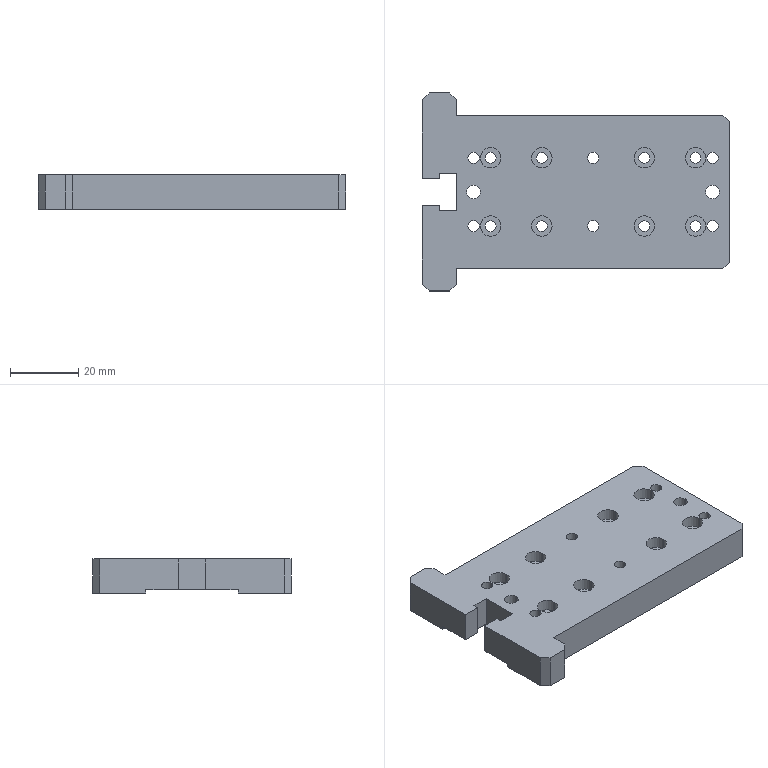Part | STEP file | PN_0050 Mount electronic clip slider mounting plate | 1 solid | 84 faces | box 90 x 58 x 10 mm | volume 36578 mm3 | cylinder 48 | plane 36 | commonest cylinder face diameters 3.2 x16 6 x16 3.3 x12 4 x4